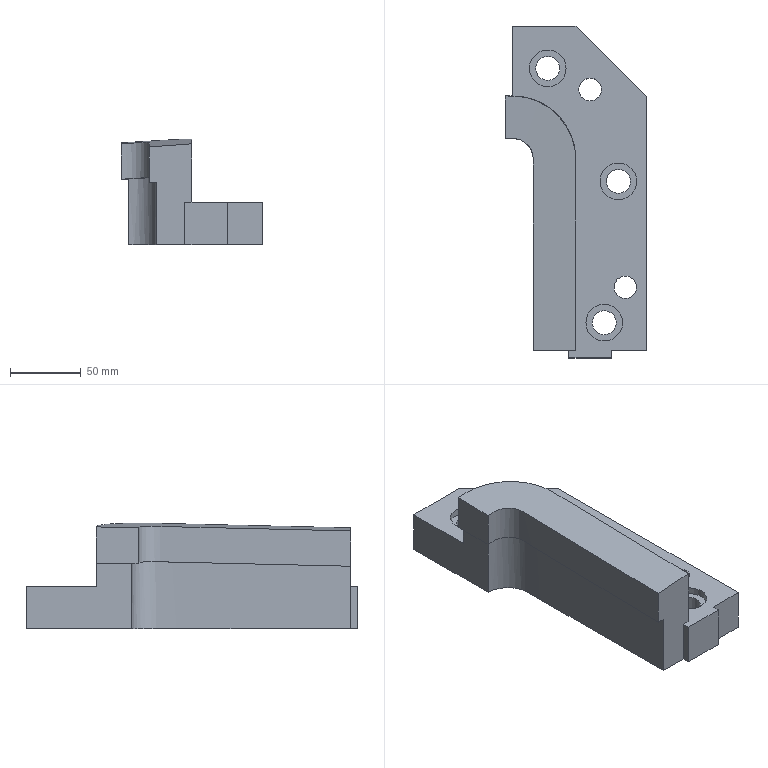Part | NX | features solid 2 | 1 solid | 30 faces | box 100.003 x 235 x 74.783 mm | volume 714230 mm3 | plane 17 | cylinder 8 | spline 5 | commonest cylinder face diameters 17 x3 26 x3 16 x2
STEP:
#1=CARTESIAN_POINT('',(660.,40.,-10.));
#2=VERTEX_POINT('',#1);
#3=CARTESIAN_POINT('',(635.,40.,-10.));
#4=VERTEX_POINT('',#3);
#5=CARTESIAN_POINT('',(660.,40.,-10.));
#6=DIRECTION('',(-1.,0.,0.));
#7=VECTOR('',#6,1000.);
#8=LINE('',#5,#7);
#9=EDGE_CURVE('',#2,#4,#8,.T.);
#10=ORIENTED_EDGE('',*,*,#9,.T.);
#11=CARTESIAN_POINT('',(635.,40.,-40.));
#12=VERTEX_POINT('',#11);
#13=CARTESIAN_POINT('',(635.,40.,-40.));
#14=DIRECTION('',(0.,0.,-1.));
#15=VECTOR('',#14,1000.);
#16=LINE('',#13,#15);
#17=EDGE_CURVE('',#12,#4,#16,.F.);
#18=ORIENTED_EDGE('',*,*,#17,.F.);
#19=CARTESIAN_POINT('',(660.,40.,-40.));
#20=VERTEX_POINT('',#19);
#21=CARTESIAN_POINT('',(609.794,40.,-40.));
#22=DIRECTION('',(-1.,0.,0.));
#23=VECTOR('',#22,1000.);
#24=LINE('',#21,#23);
#25=EDGE_CURVE('',#20,#12,#24,.T.);
#26=ORIENTED_EDGE('',*,*,#25,.F.);
#27=CARTESIAN_POINT('',(660.,40.,-300.));
#28=DIRECTION('',(0.,0.,-1.));
#29=VECTOR('',#28,1000.);
#30=LINE('',#27,#29);
#31=EDGE_CURVE('',#2,#20,#30,.T.);
#32=ORIENTED_EDGE('',*,*,#31,.F.);
#33=EDGE_LOOP('',(#10,#18,#26,#32));
#34=FACE_BOUND('',#33,.T.);
#35=CARTESIAN_POINT('',(609.803,40.,-300.));
#36=DIRECTION('',(0.,-1.,0.));
#37=DIRECTION('',(0.,0.,-1.));
#38=AXIS2_PLACEMENT_3D('',#35,#36,#37);
#39=PLANE('',#38);
#40=ADVANCED_FACE('',(#34),#39,.T.);
#41=CARTESIAN_POINT('',(605.,40.,-40.));
#42=VERTEX_POINT('',#41);
#43=CARTESIAN_POINT('',(584.803,40.,-40.));
#44=VERTEX_POINT('',#43);
#45=CARTESIAN_POINT('',(609.794,40.,-40.));
#46=DIRECTION('',(-1.,0.,0.));
#47=VECTOR('',#46,1000.);
#48=LINE('',#45,#47);
#49=EDGE_CURVE('',#42,#44,#48,.T.);
#50=ORIENTED_EDGE('',*,*,#49,.F.);
#51=CARTESIAN_POINT('',(605.,40.,-10.));
#52=VERTEX_POINT('',#51);
#53=CARTESIAN_POINT('',(605.,40.,-40.));
#54=DIRECTION('',(0.,0.,1.));
#55=VECTOR('',#54,1000.);
#56=LINE('',#53,#55);
#57=EDGE_CURVE('',#42,#52,#56,.T.);
#58=ORIENTED_EDGE('',*,*,#57,.T.);
#59=CARTESIAN_POINT('',(609.803,40.,-10.));
#60=VERTEX_POINT('',#59);
#61=CARTESIAN_POINT('',(609.803,40.,-10.));
#62=DIRECTION('',(-1.,0.,0.));
#63=VECTOR('',#62,1000.);
#64=LINE('',#61,#63);
#65=EDGE_CURVE('',#52,#60,#64,.F.);
#66=ORIENTED_EDGE('',*,*,#65,.T.);
#67=CARTESIAN_POINT('',(609.803,40.,31.479));
#68=VERTEX_POINT('',#67);
#69=CARTESIAN_POINT('',(609.803,40.,-300.));
#70=DIRECTION('',(0.,0.,1.));
#71=VECTOR('',#70,1000.);
#72=LINE('',#69,#71);
#73=EDGE_CURVE('',#60,#68,#72,.T.);
#74=ORIENTED_EDGE('',*,*,#73,.T.);
#75=CARTESIAN_POINT('',(579.803,40.,29.317));
#76=VERTEX_POINT('',#75);
#77=CARTESIAN_POINT('',(609.803,40.,31.479));
#78=CARTESIAN_POINT('',(599.805,40.,30.733));
#79=CARTESIAN_POINT('',(589.805,40.,30.013));
#80=CARTESIAN_POINT('',(579.803,40.,29.317));
#81=B_SPLINE_CURVE_WITH_KNOTS('',3,(#77,#78,#79,#80),.UNSPECIFIED.,.F.,.F.,(4,4),(0.,0.03008),.UNSPECIFIED.);
#82=EDGE_CURVE('',#68,#76,#81,.T.);
#83=ORIENTED_EDGE('',*,*,#82,.T.);
#84=CARTESIAN_POINT('',(579.803,40.,4.317));
#85=VERTEX_POINT('',#84);
#86=CARTESIAN_POINT('',(579.803,40.,-300.));
#87=DIRECTION('',(0.,0.,1.));
#88=VECTOR('',#87,1000.);
#89=LINE('',#86,#88);
#90=EDGE_CURVE('',#85,#76,#89,.T.);
#91=ORIENTED_EDGE('',*,*,#90,.F.);
#92=CARTESIAN_POINT('',(584.803,40.,4.317));
#93=VERTEX_POINT('',#92);
#94=CARTESIAN_POINT('',(584.803,40.,4.317));
#95=CARTESIAN_POINT('',(583.136,40.,4.317));
#96=CARTESIAN_POINT('',(581.47,40.,4.317));
#97=CARTESIAN_POINT('',(579.803,40.,4.317));
#98=B_SPLINE_CURVE_WITH_KNOTS('',3,(#94,#95,#96,#97),.UNSPECIFIED.,.F.,.F.,(4,4),(0.,0.005),.UNSPECIFIED.);
#99=EDGE_CURVE('',#93,#85,#98,.T.);
#100=ORIENTED_EDGE('',*,*,#99,.F.);
#101=CARTESIAN_POINT('',(584.803,40.,-145.683));
#102=DIRECTION('',(0.,0.,-1.));
#103=VECTOR('',#102,1000.);
#104=LINE('',#101,#103);
#105=EDGE_CURVE('',#44,#93,#104,.F.);
#106=ORIENTED_EDGE('',*,*,#105,.F.);
#107=EDGE_LOOP('',(#50,#58,#66,#74,#83,#91,#100,#106));
#108=FACE_BOUND('',#107,.T.);
#109=CARTESIAN_POINT('',(609.803,40.,-300.));
#110=DIRECTION('',(0.,-1.,0.));
#111=DIRECTION('',(0.,0.,-1.));
#112=AXIS2_PLACEMENT_3D('',#109,#110,#111);
#113=PLANE('',#112);
#114=ADVANCED_FACE('',(#108),#113,.T.);
#115=CARTESIAN_POINT('',(598.5,240.,-40.));
#116=VERTEX_POINT('',#115);
#117=CARTESIAN_POINT('',(590.,240.,-40.));
#118=DIRECTION('',(0.,0.,1.));
#119=DIRECTION('',(1.,0.,0.));
#120=AXIS2_PLACEMENT_3D('',#117,#118,#119);
#121=CIRCLE('',#120,8.5);
#122=EDGE_CURVE('',#116,#116,#121,.T.);
#123=ORIENTED_EDGE('',*,*,#122,.T.);
#124=EDGE_LOOP('',(#123));
#125=FACE_BOUND('',#124,.T.);
#126=CARTESIAN_POINT('',(648.5,160.,-40.));
#127=VERTEX_POINT('',#126);
#128=CARTESIAN_POINT('',(640.,160.,-40.));
#129=DIRECTION('',(0.,0.,1.));
#130=DIRECTION('',(1.,0.,0.));
#131=AXIS2_PLACEMENT_3D('',#128,#129,#130);
#132=CIRCLE('',#131,8.5);
#133=EDGE_CURVE('',#127,#127,#132,.T.);
#134=ORIENTED_EDGE('',*,*,#133,.T.);
#135=EDGE_LOOP('',(#134));
#136=FACE_BOUND('',#135,.T.);
#137=CARTESIAN_POINT('',(638.5,60.,-40.));
#138=VERTEX_POINT('',#137);
#139=CARTESIAN_POINT('',(630.,60.,-40.));
#140=DIRECTION('',(0.,0.,1.));
#141=DIRECTION('',(1.,0.,0.));
#142=AXIS2_PLACEMENT_3D('',#139,#140,#141);
#143=CIRCLE('',#142,8.5);
#144=EDGE_CURVE('',#138,#138,#143,.T.);
#145=ORIENTED_EDGE('',*,*,#144,.T.);
#146=EDGE_LOOP('',(#145));
#147=FACE_BOUND('',#146,.T.);
#148=CARTESIAN_POINT('',(628.,225.,-40.));
#149=VERTEX_POINT('',#148);
#150=CARTESIAN_POINT('',(620.,225.,-40.));
#151=DIRECTION('',(0.,0.,1.));
#152=DIRECTION('',(1.,0.,0.));
#153=AXIS2_PLACEMENT_3D('',#150,#151,#152);
#154=CIRCLE('',#153,8.);
#155=EDGE_CURVE('',#149,#149,#154,.T.);
#156=ORIENTED_EDGE('',*,*,#155,.T.);
#157=EDGE_LOOP('',(#156));
#158=FACE_BOUND('',#157,.T.);
#159=CARTESIAN_POINT('',(653.,85.,-40.));
#160=VERTEX_POINT('',#159);
#161=CARTESIAN_POINT('',(645.,85.,-40.));
#162=DIRECTION('',(0.,0.,1.));
#163=DIRECTION('',(1.,0.,0.));
#164=AXIS2_PLACEMENT_3D('',#161,#162,#163);
#165=CIRCLE('',#164,8.);
#166=EDGE_CURVE('',#160,#160,#165,.T.);
#167=ORIENTED_EDGE('',*,*,#166,.T.);
#168=EDGE_LOOP('',(#167));
#169=FACE_BOUND('',#168,.T.);
#170=CARTESIAN_POINT('',(605.,35.,-40.));
#171=VERTEX_POINT('',#170);
#172=CARTESIAN_POINT('',(605.,40.,-40.));
#173=DIRECTION('',(0.,-1.,0.));
#174=VECTOR('',#173,1000.);
#175=LINE('',#172,#174);
#176=EDGE_CURVE('',#42,#171,#175,.T.);
#177=ORIENTED_EDGE('',*,*,#176,.F.);
#178=ORIENTED_EDGE('',*,*,#49,.T.);
#179=CARTESIAN_POINT('',(565.,195.391,-40.));
#180=VERTEX_POINT('',#179);
#181=CARTESIAN_POINT('',(584.803,40.,-40.));
#182=CARTESIAN_POINT('',(584.801,46.951,-40.));
#183=CARTESIAN_POINT('',(584.798,60.853,-40.));
#184=CARTESIAN_POINT('',(584.793,81.705,-40.));
#185=CARTESIAN_POINT('',(584.79,102.558,-40.));
#186=CARTESIAN_POINT('',(584.792,119.935,-40.));
#187=CARTESIAN_POINT('',(584.798,133.836,-40.));
#188=CARTESIAN_POINT('',(584.805,144.263,-40.));
#189=CARTESIAN_POINT('',(584.816,152.951,-40.));
#190=CARTESIAN_POINT('',(584.821,159.902,-40.));
#191=CARTESIAN_POINT('',(584.836,165.116,-40.));
#192=CARTESIAN_POINT('',(584.814,170.326,-40.));
#193=CARTESIAN_POINT('',(584.936,175.551,-40.));
#194=CARTESIAN_POINT('',(584.369,180.719,-40.));
#195=CARTESIAN_POINT('',(582.328,185.559,-40.));
#196=CARTESIAN_POINT('',(579.143,189.697,-40.));
#197=CARTESIAN_POINT('',(575.018,192.889,-40.));
#198=CARTESIAN_POINT('',(570.21,194.925,-40.));
#199=CARTESIAN_POINT('',(566.731,195.341,-40.));
#200=CARTESIAN_POINT('',(565.,195.391,-40.));
#201=B_SPLINE_CURVE_WITH_KNOTS('',3,(#181,#182,#183,#184,#185,#186,#187,#188,#189,#190,#191,#192,#193,#194,#195,#196,#197,#198,#199,#200),.UNSPECIFIED.,.F.,.F.,(4,1,1,1,1,1,1,1,1,1,1,1,1,1,1,1,1,4),(0.,0.02085,0.04171,0.06256,0.08341,0.09384,0.1043,0.1147,0.1199,0.1251,0.1303,0.1355,0.1408,0.146,0.1512,0.1564,0.1616,0.1668),.UNSPECIFIED.);
#202=EDGE_CURVE('',#44,#180,#201,.T.);
#203=ORIENTED_EDGE('',*,*,#202,.T.);
#204=CARTESIAN_POINT('',(565.,270.,-40.));
#205=VERTEX_POINT('',#204);
#206=CARTESIAN_POINT('',(565.,121.934,-40.));
#207=DIRECTION('',(0.,-1.,0.));
#208=VECTOR('',#207,1000.);
#209=LINE('',#206,#208);
#210=EDGE_CURVE('',#205,#180,#209,.T.);
#211=ORIENTED_EDGE('',*,*,#210,.F.);
#212=CARTESIAN_POINT('',(610.,270.,-40.));
#213=VERTEX_POINT('',#212);
#214=CARTESIAN_POINT('',(660.,270.,-40.));
#215=DIRECTION('',(-1.,0.,0.));
#216=VECTOR('',#215,1000.);
#217=LINE('',#214,#216);
#218=EDGE_CURVE('',#213,#205,#217,.T.);
#219=ORIENTED_EDGE('',*,*,#218,.F.);
#220=CARTESIAN_POINT('',(660.,220.,-40.));
#221=VERTEX_POINT('',#220);
#222=CARTESIAN_POINT('',(660.,220.,-40.));
#223=DIRECTION('',(0.7071,-0.7071,0.));
#224=VECTOR('',#223,1000.);
#225=LINE('',#222,#224);
#226=EDGE_CURVE('',#221,#213,#225,.F.);
#227=ORIENTED_EDGE('',*,*,#226,.F.);
#228=CARTESIAN_POINT('',(660.,-215.,-40.));
#229=DIRECTION('',(0.,1.,0.));
#230=VECTOR('',#229,1000.);
#231=LINE('',#228,#230);
#232=EDGE_CURVE('',#20,#221,#231,.T.);
#233=ORIENTED_EDGE('',*,*,#232,.F.);
#234=ORIENTED_EDGE('',*,*,#25,.T.);
#235=CARTESIAN_POINT('',(635.,35.,-40.));
#236=VERTEX_POINT('',#235);
#237=CARTESIAN_POINT('',(635.,40.,-40.));
#238=DIRECTION('',(0.,1.,0.));
#239=VECTOR('',#238,1000.);
#240=LINE('',#237,#239);
#241=EDGE_CURVE('',#12,#236,#240,.F.);
#242=ORIENTED_EDGE('',*,*,#241,.T.);
#243=CARTESIAN_POINT('',(645.,35.,-40.));
#244=DIRECTION('',(1.,0.,0.));
#245=VECTOR('',#244,1000.);
#246=LINE('',#243,#245);
#247=EDGE_CURVE('',#236,#171,#246,.F.);
#248=ORIENTED_EDGE('',*,*,#247,.T.);
#249=EDGE_LOOP('',(#177,#178,#203,#211,#219,#227,#233,#234,#242,#248));
#250=FACE_BOUND('',#249,.T.);
#251=CARTESIAN_POINT('',(609.794,121.934,-40.));
#252=DIRECTION('',(0.,0.,1.));
#253=DIRECTION('',(-1.,0.,0.));
#254=AXIS2_PLACEMENT_3D('',#251,#252,#253);
#255=PLANE('',#254);
#256=ADVANCED_FACE('',(#125,#136,#147,#158,#169,#250),#255,.F.);
#257=CARTESIAN_POINT('',(603.,240.,-10.));
#258=VERTEX_POINT('',#257);
#259=CARTESIAN_POINT('',(590.,240.,-10.));
#260=DIRECTION('',(0.,0.,1.));
#261=DIRECTION('',(1.,0.,0.));
#262=AXIS2_PLACEMENT_3D('',#259,#260,#261);
#263=CIRCLE('',#262,13.);
#264=EDGE_CURVE('',#258,#258,#263,.T.);
#265=ORIENTED_EDGE('',*,*,#264,.F.);
#266=EDGE_LOOP('',(#265));
#267=FACE_BOUND('',#266,.T.);
#268=CARTESIAN_POINT('',(653.,160.,-10.));
#269=VERTEX_POINT('',#268);
#270=CARTESIAN_POINT('',(640.,160.,-10.));
#271=DIRECTION('',(0.,0.,1.));
#272=DIRECTION('',(1.,0.,0.));
#273=AXIS2_PLACEMENT_3D('',#270,#271,#272);
#274=CIRCLE('',#273,13.);
#275=EDGE_CURVE('',#269,#269,#274,.T.);
#276=ORIENTED_EDGE('',*,*,#275,.F.);
#277=EDGE_LOOP('',(#276));
#278=FACE_BOUND('',#277,.T.);
#279=CARTESIAN_POINT('',(643.,60.,-10.));
#280=VERTEX_POINT('',#279);
#281=CARTESIAN_POINT('',(630.,60.,-10.));
#282=DIRECTION('',(0.,0.,1.));
#283=DIRECTION('',(1.,0.,0.));
#284=AXIS2_PLACEMENT_3D('',#281,#282,#283);
#285=CIRCLE('',#284,13.);
#286=EDGE_CURVE('',#280,#280,#285,.T.);
#287=ORIENTED_EDGE('',*,*,#286,.F.);
#288=EDGE_LOOP('',(#287));
#289=FACE_BOUND('',#288,.T.);
#290=CARTESIAN_POINT('',(628.,225.,-10.));
#291=VERTEX_POINT('',#290);
#292=CARTESIAN_POINT('',(620.,225.,-10.));
#293=DIRECTION('',(0.,0.,1.));
#294=DIRECTION('',(1.,0.,0.));
#295=AXIS2_PLACEMENT_3D('',#292,#293,#294);
#296=CIRCLE('',#295,8.);
#297=EDGE_CURVE('',#291,#291,#296,.T.);
#298=ORIENTED_EDGE('',*,*,#297,.F.);
#299=EDGE_LOOP('',(#298));
#300=FACE_BOUND('',#299,.T.);
#301=CARTESIAN_POINT('',(653.,85.,-10.));
#302=VERTEX_POINT('',#301);
#303=CARTESIAN_POINT('',(645.,85.,-10.));
#304=DIRECTION('',(0.,0.,1.));
#305=DIRECTION('',(1.,0.,0.));
#306=AXIS2_PLACEMENT_3D('',#303,#304,#305);
#307=CIRCLE('',#306,8.);
#308=EDGE_CURVE('',#302,#302,#307,.T.);
#309=ORIENTED_EDGE('',*,*,#308,.F.);
#310=EDGE_LOOP('',(#309));
#311=FACE_BOUND('',#310,.T.);
#312=CARTESIAN_POINT('',(635.,35.,-10.));
#313=VERTEX_POINT('',#312);
#314=CARTESIAN_POINT('',(635.,40.,-10.));
#315=DIRECTION('',(0.,-1.,0.));
#316=VECTOR('',#315,1000.);
#317=LINE('',#314,#316);
#318=EDGE_CURVE('',#4,#313,#317,.T.);
#319=ORIENTED_EDGE('',*,*,#318,.F.);
#320=ORIENTED_EDGE('',*,*,#9,.F.);
#321=CARTESIAN_POINT('',(660.,220.,-10.));
#322=VERTEX_POINT('',#321);
#323=CARTESIAN_POINT('',(660.,-215.,-10.));
#324=DIRECTION('',(0.,1.,0.));
#325=VECTOR('',#324,1000.);
#326=LINE('',#323,#325);
#327=EDGE_CURVE('',#2,#322,#326,.T.);
#328=ORIENTED_EDGE('',*,*,#327,.T.);
#329=CARTESIAN_POINT('',(610.,270.,-10.));
#330=VERTEX_POINT('',#329);
#331=CARTESIAN_POINT('',(877.5,2.5,-10.));
#332=DIRECTION('',(-0.7071,0.7071,0.));
#333=VECTOR('',#332,1000.);
#334=LINE('',#331,#333);
#335=EDGE_CURVE('',#330,#322,#334,.F.);
#336=ORIENTED_EDGE('',*,*,#335,.F.);
#337=CARTESIAN_POINT('',(565.,270.,-10.));
#338=VERTEX_POINT('',#337);
#339=CARTESIAN_POINT('',(660.,270.,-10.));
#340=DIRECTION('',(-1.,0.,0.));
#341=VECTOR('',#340,1000.);
#342=LINE('',#339,#341);
#343=EDGE_CURVE('',#330,#338,#342,.T.);
#344=ORIENTED_EDGE('',*,*,#343,.T.);
#345=CARTESIAN_POINT('',(565.,220.388,-10.));
#346=VERTEX_POINT('',#345);
#347=CARTESIAN_POINT('',(565.,-215.,-10.));
#348=DIRECTION('',(0.,-1.,0.));
#349=VECTOR('',#348,1000.);
#350=LINE('',#347,#349);
#351=EDGE_CURVE('',#338,#346,#350,.T.);
#352=ORIENTED_EDGE('',*,*,#351,.T.);
#353=CARTESIAN_POINT('',(609.803,40.,-10.));
#354=CARTESIAN_POINT('',(609.797,67.324,-10.));
#355=CARTESIAN_POINT('',(609.766,108.793,-10.));
#356=CARTESIAN_POINT('',(609.827,152.054,-10.));
#357=CARTESIAN_POINT('',(609.828,170.484,-10.));
#358=CARTESIAN_POINT('',(609.852,174.233,-10.));
#359=CARTESIAN_POINT('',(609.824,176.995,-10.));
#360=CARTESIAN_POINT('',(609.6,180.207,-10.));
#361=CARTESIAN_POINT('',(608.89,185.117,-10.));
#362=CARTESIAN_POINT('',(607.115,191.421,-10.));
#363=CARTESIAN_POINT('',(603.789,198.368,-10.));
#364=CARTESIAN_POINT('',(599.387,204.588,-10.));
#365=CARTESIAN_POINT('',(593.924,210.044,-10.));
#366=CARTESIAN_POINT('',(587.673,214.455,-10.));
#367=CARTESIAN_POINT('',(580.59,217.807,-10.));
#368=CARTESIAN_POINT('',(573.327,219.802,-10.));
#369=CARTESIAN_POINT('',(568.272,220.327,-10.));
#370=CARTESIAN_POINT('',(565.167,220.389,-10.));
#371=CARTESIAN_POINT('',(564.525,220.39,-10.));
#372=CARTESIAN_POINT('',(563.605,220.383,-10.));
#373=CARTESIAN_POINT('',(562.153,220.388,-10.));
#374=CARTESIAN_POINT('',(560.855,220.386,-10.));
#375=CARTESIAN_POINT('',(560.,220.386,-10.));
#376=B_SPLINE_CURVE_WITH_KNOTS('',3,(#353,#354,#355,#356,#357,#358,#359,#360,#361,#362,#363,#364,#365,#366,#367,#368,#369,#370,#371,#372,#373,#374,#375),.UNSPECIFIED.,.F.,.F.,(4,1,1,1,1,1,1,1,1,1,1,1,1,1,1,1,1,1,1,1,4),(0.,0.5,0.75,0.8125,0.8203,0.8281,0.8359,0.8437,0.8594,0.875,0.8906,0.9062,0.9218,0.9375,0.9531,0.9677,0.9687,0.9726,0.9765,0.9843,1.),.UNSPECIFIED.);
#377=EDGE_CURVE('',#346,#60,#376,.F.);
#378=ORIENTED_EDGE('',*,*,#377,.T.);
#379=ORIENTED_EDGE('',*,*,#65,.F.);
#380=CARTESIAN_POINT('',(605.,35.,-10.));
#381=VERTEX_POINT('',#380);
#382=CARTESIAN_POINT('',(605.,40.,-10.));
#383=DIRECTION('',(0.,1.,0.));
#384=VECTOR('',#383,1000.);
#385=LINE('',#382,#384);
#386=EDGE_CURVE('',#52,#381,#385,.F.);
#387=ORIENTED_EDGE('',*,*,#386,.T.);
#388=CARTESIAN_POINT('',(645.,35.,-10.));
#389=DIRECTION('',(1.,0.,0.));
#390=VECTOR('',#389,1000.);
#391=LINE('',#388,#390);
#392=EDGE_CURVE('',#313,#381,#391,.F.);
#393=ORIENTED_EDGE('',*,*,#392,.F.);
#394=EDGE_LOOP('',(#319,#320,#328,#336,#344,#352,#378,#379,#387,#393));
#395=FACE_BOUND('',#394,.T.);
#396=CARTESIAN_POINT('',(660.,-215.,-10.));
#397=DIRECTION('',(0.,0.,1.));
#398=DIRECTION('',(0.,1.,0.));
#399=AXIS2_PLACEMENT_3D('',#396,#397,#398);
#400=PLANE('',#399);
#401=ADVANCED_FACE('',(#267,#278,#289,#300,#311,#395),#400,.T.);
#402=CARTESIAN_POINT('',(560.,220.386,6.411));
#403=VERTEX_POINT('',#402);
#404=CARTESIAN_POINT('',(565.,220.388,6.411));
#405=VERTEX_POINT('',#404);
#406=CARTESIAN_POINT('',(609.803,40.,6.411));
#407=CARTESIAN_POINT('',(609.797,67.324,6.411));
#408=CARTESIAN_POINT('',(609.766,108.793,6.411));
#409=CARTESIAN_POINT('',(609.827,152.054,6.411));
#410=CARTESIAN_POINT('',(609.828,170.484,6.411));
#411=CARTESIAN_POINT('',(609.852,174.233,6.411));
#412=CARTESIAN_POINT('',(609.824,176.995,6.411));
#413=CARTESIAN_POINT('',(609.6,180.207,6.411));
#414=CARTESIAN_POINT('',(608.89,185.117,6.411));
#415=CARTESIAN_POINT('',(607.115,191.421,6.411));
#416=CARTESIAN_POINT('',(603.789,198.368,6.411));
#417=CARTESIAN_POINT('',(599.387,204.588,6.411));
#418=CARTESIAN_POINT('',(593.924,210.044,6.411));
#419=CARTESIAN_POINT('',(587.673,214.455,6.411));
#420=CARTESIAN_POINT('',(580.59,217.807,6.411));
#421=CARTESIAN_POINT('',(573.327,219.802,6.411));
#422=CARTESIAN_POINT('',(568.272,220.327,6.411));
#423=CARTESIAN_POINT('',(565.167,220.389,6.411));
#424=CARTESIAN_POINT('',(564.525,220.39,6.411));
#425=CARTESIAN_POINT('',(563.605,220.383,6.411));
#426=CARTESIAN_POINT('',(562.153,220.388,6.411));
#427=CARTESIAN_POINT('',(560.855,220.386,6.411));
#428=CARTESIAN_POINT('',(560.,220.386,6.411));
#429=B_SPLINE_CURVE_WITH_KNOTS('',3,(#406,#407,#408,#409,#410,#411,#412,#413,#414,#415,#416,#417,#418,#419,#420,#421,#422,#423,#424,#425,#426,#427,#428),.UNSPECIFIED.,.F.,.F.,(4,1,1,1,1,1,1,1,1,1,1,1,1,1,1,1,1,1,1,1,4),(0.,0.5,0.75,0.8125,0.8203,0.8281,0.8359,0.8437,0.8594,0.875,0.8906,0.9062,0.9218,0.9375,0.9531,0.9677,0.9687,0.9726,0.9765,0.9843,1.),.UNSPECIFIED.);
#430=EDGE_CURVE('',#403,#405,#429,.F.);
#431=ORIENTED_EDGE('',*,*,#430,.F.);
#432=CARTESIAN_POINT('',(560.,220.386,32.162));
#433=VERTEX_POINT('',#432);
#434=CARTESIAN_POINT('',(560.,220.386,-300.));
#435=DIRECTION('',(0.,0.,1.));
#436=VECTOR('',#435,1000.);
#437=LINE('',#434,#436);
#438=EDGE_CURVE('',#403,#433,#437,.T.);
#439=ORIENTED_EDGE('',*,*,#438,.T.);
#440=CARTESIAN_POINT('',(609.803,40.,31.479));
#441=CARTESIAN_POINT('',(609.801,48.812,31.683));
#442=CARTESIAN_POINT('',(609.794,66.437,32.092));
#443=CARTESIAN_POINT('',(609.785,92.875,32.705));
#444=CARTESIAN_POINT('',(609.788,114.906,33.217));
#445=CARTESIAN_POINT('',(609.803,132.531,33.627));
#446=CARTESIAN_POINT('',(609.815,145.75,33.935));
#447=CARTESIAN_POINT('',(609.826,156.765,34.191));
#448=CARTESIAN_POINT('',(609.825,165.579,34.396));
#449=CARTESIAN_POINT('',(609.842,172.184,34.551));
#450=CARTESIAN_POINT('',(609.852,178.808,34.705));
#451=CARTESIAN_POINT('',(608.888,185.257,34.783));
#452=CARTESIAN_POINT('',(606.977,191.607,34.788));
#453=CARTESIAN_POINT('',(604.197,197.54,34.721));
#454=CARTESIAN_POINT('',(600.586,203.017,34.583));
#455=CARTESIAN_POINT('',(596.16,207.944,34.376));
#456=CARTESIAN_POINT('',(591.163,212.123,34.113));
#457=CARTESIAN_POINT('',(585.484,215.58,33.791));
#458=CARTESIAN_POINT('',(579.498,218.127,33.431));
#459=CARTESIAN_POINT('',(573.089,219.808,33.028));
#460=CARTESIAN_POINT('',(566.568,220.498,32.602));
#461=CARTESIAN_POINT('',(562.187,220.386,32.307));
#462=CARTESIAN_POINT('',(560.,220.386,32.162));
#463=B_SPLINE_CURVE_WITH_KNOTS('',3,(#440,#441,#442,#443,#444,#445,#446,#447,#448,#449,#450,#451,#452,#453,#454,#455,#456,#457,#458,#459,#460,#461,#462),.UNSPECIFIED.,.F.,.F.,(4,1,1,1,1,1,1,1,1,1,1,1,1,1,1,1,1,1,1,1,4),(0.,0.02644,0.05289,0.07933,0.09256,0.1058,0.119,0.1256,0.1322,0.1388,0.1454,0.1521,0.1587,0.1653,0.1719,0.1785,0.1851,0.1917,0.1983,0.2049,0.2116),.UNSPECIFIED.);
#464=EDGE_CURVE('',#68,#433,#463,.T.);
#465=ORIENTED_EDGE('',*,*,#464,.F.);
#466=ORIENTED_EDGE('',*,*,#73,.F.);
#467=ORIENTED_EDGE('',*,*,#377,.F.);
#468=CARTESIAN_POINT('',(565.,220.388,12.531));
#469=DIRECTION('',(0.,0.,1.));
#470=VECTOR('',#469,1000.);
#471=LINE('',#468,#470);
#472=EDGE_CURVE('',#405,#346,#471,.F.);
#473=ORIENTED_EDGE('',*,*,#472,.F.);
#474=EDGE_LOOP('',(#431,#439,#465,#466,#467,#473));
#475=FACE_BOUND('',#474,.T.);
#476=CARTESIAN_POINT('',(609.803,40.,-10.));
#477=CARTESIAN_POINT('',(609.803,40.,35.062));
#478=CARTESIAN_POINT('',(609.798,63.909,-10.));
#479=CARTESIAN_POINT('',(609.798,63.909,35.062));
#480=CARTESIAN_POINT('',(609.779,91.515,-10.));
#481=CARTESIAN_POINT('',(609.779,91.515,35.062));
#482=CARTESIAN_POINT('',(609.796,127.017,-10.));
#483=CARTESIAN_POINT('',(609.796,127.017,35.062));
#484=CARTESIAN_POINT('',(609.811,140.392,-10.));
#485=CARTESIAN_POINT('',(609.811,140.392,35.062));
#486=CARTESIAN_POINT('',(609.821,152.406,-10.));
#487=CARTESIAN_POINT('',(609.821,152.406,35.062));
#488=CARTESIAN_POINT('',(609.824,156.744,-10.));
#489=CARTESIAN_POINT('',(609.824,156.744,35.062));
#490=CARTESIAN_POINT('',(609.826,160.248,-10.));
#491=CARTESIAN_POINT('',(609.826,160.248,35.062));
#492=CARTESIAN_POINT('',(609.827,162.895,-10.));
#493=CARTESIAN_POINT('',(609.827,162.895,35.062));
#494=CARTESIAN_POINT('',(609.828,165.562,-10.));
#495=CARTESIAN_POINT('',(609.828,165.562,35.062));
#496=CARTESIAN_POINT('',(609.83,168.194,-10.));
#497=CARTESIAN_POINT('',(609.83,168.194,35.062));
#498=CARTESIAN_POINT('',(609.834,170.313,-10.));
#499=CARTESIAN_POINT('',(609.834,170.313,35.062));
#500=CARTESIAN_POINT('',(609.84,171.936,-10.));
#501=CARTESIAN_POINT('',(609.84,171.936,35.062));
#502=CARTESIAN_POINT('',(609.845,173.11,-10.));
#503=CARTESIAN_POINT('',(609.845,173.11,35.062));
#504=CARTESIAN_POINT('',(609.852,174.237,-10.));
#505=CARTESIAN_POINT('',(609.852,174.237,35.062));
#506=CARTESIAN_POINT('',(609.824,177.003,-10.));
#507=CARTESIAN_POINT('',(609.824,177.003,35.062));
#508=CARTESIAN_POINT('',(609.599,180.216,-10.));
#509=CARTESIAN_POINT('',(609.599,180.216,35.062));
#510=CARTESIAN_POINT('',(608.888,185.127,-10.));
#511=CARTESIAN_POINT('',(608.888,185.127,35.062));
#512=CARTESIAN_POINT('',(607.111,191.431,-10.));
#513=CARTESIAN_POINT('',(607.111,191.431,35.062));
#514=CARTESIAN_POINT('',(603.783,198.377,-10.));
#515=CARTESIAN_POINT('',(603.783,198.377,35.062));
#516=CARTESIAN_POINT('',(599.379,204.596,-10.));
#517=CARTESIAN_POINT('',(599.379,204.596,35.062));
#518=CARTESIAN_POINT('',(593.914,210.052,-10.));
#519=CARTESIAN_POINT('',(593.914,210.052,35.062));
#520=CARTESIAN_POINT('',(587.662,214.461,-10.));
#521=CARTESIAN_POINT('',(587.662,214.461,35.062));
#522=CARTESIAN_POINT('',(581.758,217.253,-10.));
#523=CARTESIAN_POINT('',(581.758,217.253,35.062));
#524=CARTESIAN_POINT('',(576.868,218.83,-10.));
#525=CARTESIAN_POINT('',(576.868,218.83,35.062));
#526=CARTESIAN_POINT('',(573.76,219.543,-10.));
#527=CARTESIAN_POINT('',(573.76,219.543,35.062));
#528=CARTESIAN_POINT('',(571.251,219.953,-10.));
#529=CARTESIAN_POINT('',(571.251,219.953,35.062));
#530=CARTESIAN_POINT('',(569.369,220.179,-10.));
#531=CARTESIAN_POINT('',(569.369,220.179,35.062));
#532=CARTESIAN_POINT('',(567.793,220.301,-10.));
#533=CARTESIAN_POINT('',(567.793,220.301,35.062));
#534=CARTESIAN_POINT('',(566.562,220.359,-10.));
#535=CARTESIAN_POINT('',(566.562,220.359,35.062));
#536=CARTESIAN_POINT('',(565.248,220.389,-10.));
#537=CARTESIAN_POINT('',(565.248,220.389,35.062));
#538=CARTESIAN_POINT('',(564.514,220.39,-10.));
#539=CARTESIAN_POINT('',(564.514,220.39,35.062));
#540=CARTESIAN_POINT('',(563.603,220.383,-10.));
#541=CARTESIAN_POINT('',(563.603,220.383,35.062));
#542=CARTESIAN_POINT('',(562.563,220.386,-10.));
#543=CARTESIAN_POINT('',(562.563,220.386,35.062));
#544=CARTESIAN_POINT('',(561.286,220.387,-10.));
#545=CARTESIAN_POINT('',(561.286,220.387,35.062));
#546=CARTESIAN_POINT('',(560.427,220.386,-10.));
#547=CARTESIAN_POINT('',(560.427,220.386,35.062));
#548=CARTESIAN_POINT('',(560.,220.386,-10.));
#549=CARTESIAN_POINT('',(560.,220.386,35.062));
#550=B_SPLINE_SURFACE_WITH_KNOTS('',3,1,((#476,#477),(#478,#479),(#480,#481),(#482,#483),(#484,#485),(#486,#487),(#488,#489),(#490,#491),(#492,#493),(#494,#495),(#496,#497),(#498,#499),(#500,#501),(#502,#503),(#504,#505),(#506,#507),(#508,#509),(#510,#511),(#512,#513),(#514,#515),(#516,#517),(#518,#519),(#520,#521),(#522,#523),(#524,#525),(#526,#527),(#528,#529),(#530,#531),(#532,#533),(#534,#535),(#536,#537),(#538,#539),(#540,#541),(#542,#543),(#544,#545),(#546,#547),(#548,#549)),.UNSPECIFIED.,.F.,.F.,.F.,(4,1,1,1,1,1,1,1,1,1,1,1,1,1,1,1,1,1,1,1,1,1,1,1,1,1,1,1,1,1,1,1,1,1,4),(2,2),(0.,0.4375,0.5,0.6562,0.6875,0.7188,0.7344,0.75,0.7656,0.7812,0.7969,0.8047,0.8125,0.8203,0.8281,0.8359,0.8438,0.8594,0.875,0.8906,0.9062,0.9219,0.9375,0.9453,0.9531,0.957,0.9609,0.9648,0.9668,0.9688,0.9727,0.9766,0.9844,0.9922,1.),(0.,1.),.UNSPECIFIED.);
#551=ADVANCED_FACE('',(#475),#550,.T.);
#552=ORIENTED_EDGE('',*,*,#218,.T.);
#553=CARTESIAN_POINT('',(565.,270.,6.411));
#554=DIRECTION('',(0.,0.,-1.));
#555=VECTOR('',#554,1000.);
#556=LINE('',#553,#555);
#557=EDGE_CURVE('',#338,#205,#556,.T.);
#558=ORIENTED_EDGE('',*,*,#557,.F.);
#559=ORIENTED_EDGE('',*,*,#343,.F.);
#560=CARTESIAN_POINT('',(610.,270.,-10.));
#561=DIRECTION('',(0.,0.,1.));
#562=VECTOR('',#561,1000.);
#563=LINE('',#560,#562);
#564=EDGE_CURVE('',#213,#330,#563,.T.);
#565=ORIENTED_EDGE('',*,*,#564,.F.);
#566=EDGE_LOOP('',(#552,#558,#559,#565));
#567=FACE_BOUND('',#566,.T.);
#568=CARTESIAN_POINT('',(660.,270.,-10.));
#569=DIRECTION('',(0.,1.,0.));
#570=DIRECTION('',(0.,0.,-1.));
#571=AXIS2_PLACEMENT_3D('',#568,#569,#570);
#572=PLANE('',#571);
#573=ADVANCED_FACE('',(#567),#572,.T.);
#574=CARTESIAN_POINT('',(560.,190.386,6.411));
#575=VERTEX_POINT('',#574);
#576=CARTESIAN_POINT('',(559.997,195.387,6.411));
#577=VERTEX_POINT('',#576);
#578=CARTESIAN_POINT('',(560.,190.386,6.411));
#579=DIRECTION('',(0.,1.,0.));
#580=VECTOR('',#579,1000.);
#581=LINE('',#578,#580);
#582=EDGE_CURVE('',#575,#577,#581,.T.);
#583=ORIENTED_EDGE('',*,*,#582,.F.);
#584=CARTESIAN_POINT('',(560.,190.386,31.465));
#585=VERTEX_POINT('',#584);
#586=CARTESIAN_POINT('',(560.,190.386,-300.));
#587=DIRECTION('',(0.,0.,1.));
#588=VECTOR('',#587,1000.);
#589=LINE('',#586,#588);
#590=EDGE_CURVE('',#575,#585,#589,.T.);
#591=ORIENTED_EDGE('',*,*,#590,.T.);
#592=CARTESIAN_POINT('',(560.,190.386,31.465));
#593=CARTESIAN_POINT('',(560.,200.386,31.698));
#594=CARTESIAN_POINT('',(560.,210.386,31.93));
#595=CARTESIAN_POINT('',(560.,220.386,32.162));
#596=B_SPLINE_CURVE_WITH_KNOTS('',3,(#592,#593,#594,#595),.UNSPECIFIED.,.F.,.F.,(4,4),(0.,0.03001),.UNSPECIFIED.);
#597=EDGE_CURVE('',#585,#433,#596,.T.);
#598=ORIENTED_EDGE('',*,*,#597,.T.);
#599=ORIENTED_EDGE('',*,*,#438,.F.);
#600=CARTESIAN_POINT('',(560.,190.386,6.411));
#601=DIRECTION('',(0.,1.,0.));
#602=VECTOR('',#601,1000.);
#603=LINE('',#600,#602);
#604=EDGE_CURVE('',#577,#403,#603,.T.);
#605=ORIENTED_EDGE('',*,*,#604,.F.);
#606=EDGE_LOOP('',(#583,#591,#598,#599,#605));
#607=FACE_BOUND('',#606,.T.);
#608=CARTESIAN_POINT('',(560.,190.386,-300.));
#609=DIRECTION('',(-1.,0.,0.));
#610=DIRECTION('',(0.,0.,-1.));
#611=AXIS2_PLACEMENT_3D('',#608,#609,#610);
#612=PLANE('',#611);
#613=ADVANCED_FACE('',(#607),#612,.T.);
#614=CARTESIAN_POINT('',(579.803,40.,4.317));
#615=CARTESIAN_POINT('',(579.801,46.829,4.421));
#616=CARTESIAN_POINT('',(579.798,60.482,4.808));
#617=CARTESIAN_POINT('',(579.794,80.964,5.255));
#618=CARTESIAN_POINT('',(579.791,101.446,5.738));
#619=CARTESIAN_POINT('',(579.792,118.515,6.133));
#620=CARTESIAN_POINT('',(579.797,132.17,6.45));
#621=CARTESIAN_POINT('',(579.803,142.41,6.688));
#622=CARTESIAN_POINT('',(579.813,152.652,6.927));
#623=CARTESIAN_POINT('',(579.824,161.184,7.125));
#624=CARTESIAN_POINT('',(579.835,168.016,7.285));
#625=CARTESIAN_POINT('',(579.845,173.122,7.402));
#626=CARTESIAN_POINT('',(579.853,178.297,7.532));
#627=CARTESIAN_POINT('',(578.02,183.147,7.517));
#628=CARTESIAN_POINT('',(574.704,187.111,7.36));
#629=CARTESIAN_POINT('',(570.97,189.292,7.138));
#630=CARTESIAN_POINT('',(567.696,190.203,6.923));
#631=CARTESIAN_POINT('',(565.139,190.431,6.752));
#632=CARTESIAN_POINT('',(562.568,190.373,6.58));
#633=CARTESIAN_POINT('',(560.856,190.386,6.467));
#634=CARTESIAN_POINT('',(560.,190.386,6.411));
#635=B_SPLINE_CURVE_WITH_KNOTS('',3,(#614,#615,#616,#617,#618,#619,#620,#621,#622,#623,#624,#625,#626,#627,#628,#629,#630,#631,#632,#633,#634),.UNSPECIFIED.,.F.,.F.,(4,1,1,1,1,1,1,1,1,1,1,1,1,1,1,1,1,1,4),(0.,0.02049,0.04098,0.06146,0.08195,0.09219,0.1024,0.1127,0.1229,0.128,0.1332,0.1383,0.1434,0.1485,0.1537,0.1562,0.1588,0.1613,0.1639),.UNSPECIFIED.);
#636=EDGE_CURVE('',#85,#575,#635,.T.);
#637=ORIENTED_EDGE('',*,*,#636,.F.);
#638=ORIENTED_EDGE('',*,*,#90,.T.);
#639=CARTESIAN_POINT('',(579.803,40.,29.317));
#640=CARTESIAN_POINT('',(579.801,46.811,29.475));
#641=CARTESIAN_POINT('',(579.798,60.433,29.792));
#642=CARTESIAN_POINT('',(579.794,80.866,30.266));
#643=CARTESIAN_POINT('',(579.791,101.3,30.74));
#644=CARTESIAN_POINT('',(579.792,118.327,31.135));
#645=CARTESIAN_POINT('',(579.797,131.949,31.452));
#646=CARTESIAN_POINT('',(579.803,142.166,31.689));
#647=CARTESIAN_POINT('',(579.813,152.382,31.927));
#648=CARTESIAN_POINT('',(579.821,160.896,32.126));
#649=CARTESIAN_POINT('',(579.838,167.707,32.285));
#650=CARTESIAN_POINT('',(579.829,172.816,32.403));
#651=CARTESIAN_POINT('',(579.909,177.922,32.527));
#652=CARTESIAN_POINT('',(578.17,182.922,32.522));
#653=CARTESIAN_POINT('',(574.838,187.005,32.387));
#654=CARTESIAN_POINT('',(571.08,189.254,32.182));
#655=CARTESIAN_POINT('',(567.719,190.202,31.977));
#656=CARTESIAN_POINT('',(565.15,190.432,31.809));
#657=CARTESIAN_POINT('',(562.574,190.373,31.636));
#658=CARTESIAN_POINT('',(560.858,190.386,31.522));
#659=CARTESIAN_POINT('',(560.,190.386,31.465));
#660=B_SPLINE_CURVE_WITH_KNOTS('',3,(#639,#640,#641,#642,#643,#644,#645,#646,#647,#648,#649,#650,#651,#652,#653,#654,#655,#656,#657,#658,#659),.UNSPECIFIED.,.F.,.F.,(4,1,1,1,1,1,1,1,1,1,1,1,1,1,1,1,1,1,4),(0.,0.02044,0.04088,0.06132,0.08175,0.09197,0.1022,0.1124,0.1226,0.1277,0.1329,0.138,0.1431,0.1482,0.1533,0.1558,0.1584,0.161,0.1635),.UNSPECIFIED.);
#661=EDGE_CURVE('',#76,#585,#660,.T.);
#662=ORIENTED_EDGE('',*,*,#661,.T.);
#663=ORIENTED_EDGE('',*,*,#590,.F.);
#664=EDGE_LOOP('',(#637,#638,#662,#663));
#665=FACE_BOUND('',#664,.T.);
#666=CARTESIAN_POINT('',(579.803,40.,4.148));
#667=CARTESIAN_POINT('',(579.803,40.,32.689));
#668=CARTESIAN_POINT('',(579.801,46.83,4.148));
#669=CARTESIAN_POINT('',(579.801,46.83,32.689));
#670=CARTESIAN_POINT('',(579.798,60.49,4.148));
#671=CARTESIAN_POINT('',(579.798,60.49,32.689));
#672=CARTESIAN_POINT('',(579.794,80.98,4.148));
#673=CARTESIAN_POINT('',(579.794,80.98,32.689));
#674=CARTESIAN_POINT('',(579.791,101.47,4.148));
#675=CARTESIAN_POINT('',(579.791,101.47,32.689));
#676=CARTESIAN_POINT('',(579.792,118.545,4.148));
#677=CARTESIAN_POINT('',(579.792,118.545,32.689));
#678=CARTESIAN_POINT('',(579.797,132.205,4.148));
#679=CARTESIAN_POINT('',(579.797,132.205,32.689));
#680=CARTESIAN_POINT('',(579.803,142.449,4.148));
#681=CARTESIAN_POINT('',(579.803,142.449,32.689));
#682=CARTESIAN_POINT('',(579.813,152.695,4.148));
#683=CARTESIAN_POINT('',(579.813,152.695,32.689));
#684=CARTESIAN_POINT('',(579.824,161.23,4.148));
#685=CARTESIAN_POINT('',(579.824,161.23,32.689));
#686=CARTESIAN_POINT('',(579.834,168.064,4.148));
#687=CARTESIAN_POINT('',(579.834,168.064,32.689));
#688=CARTESIAN_POINT('',(579.847,173.175,4.148));
#689=CARTESIAN_POINT('',(579.847,173.175,32.689));
#690=CARTESIAN_POINT('',(579.847,178.34,4.148));
#691=CARTESIAN_POINT('',(579.847,178.34,32.689));
#692=CARTESIAN_POINT('',(577.991,183.196,4.148));
#693=CARTESIAN_POINT('',(577.991,183.196,32.689));
#694=CARTESIAN_POINT('',(574.673,187.132,4.148));
#695=CARTESIAN_POINT('',(574.673,187.132,32.689));
#696=CARTESIAN_POINT('',(570.966,189.295,4.148));
#697=CARTESIAN_POINT('',(570.966,189.295,32.689));
#698=CARTESIAN_POINT('',(567.676,190.208,4.148));
#699=CARTESIAN_POINT('',(567.676,190.208,32.689));
#700=CARTESIAN_POINT('',(565.121,190.431,4.148));
#701=CARTESIAN_POINT('',(565.121,190.431,32.689));
#702=CARTESIAN_POINT('',(562.56,190.373,4.148));
#703=CARTESIAN_POINT('',(562.56,190.373,32.689));
#704=CARTESIAN_POINT('',(560.853,190.386,4.148));
#705=CARTESIAN_POINT('',(560.853,190.386,32.689));
#706=CARTESIAN_POINT('',(560.,190.386,4.148));
#707=CARTESIAN_POINT('',(560.,190.386,32.689));
#708=B_SPLINE_SURFACE_WITH_KNOTS('',3,1,((#666,#667),(#668,#669),(#670,#671),(#672,#673),(#674,#675),(#676,#677),(#678,#679),(#680,#681),(#682,#683),(#684,#685),(#686,#687),(#688,#689),(#690,#691),(#692,#693),(#694,#695),(#696,#697),(#698,#699),(#700,#701),(#702,#703),(#704,#705),(#706,#707)),.SURF_OF_LINEAR_EXTRUSION.,.F.,.F.,.F.,(4,1,1,1,1,1,1,1,1,1,1,1,1,1,1,1,1,1,4),(2,2),(0.,0.125,0.25,0.375,0.5,0.5625,0.625,0.6875,0.75,0.7812,0.8125,0.8438,0.875,0.9062,0.9375,0.9531,0.9688,0.9844,1.),(0.,1.),.UNSPECIFIED.);
#709=ADVANCED_FACE('',(#665),#708,.F.);
#710=ORIENTED_EDGE('',*,*,#82,.F.);
#711=ORIENTED_EDGE('',*,*,#464,.T.);
#712=ORIENTED_EDGE('',*,*,#597,.F.);
#713=ORIENTED_EDGE('',*,*,#661,.F.);
#714=EDGE_LOOP('',(#710,#711,#712,#713));
#715=FACE_BOUND('',#714,.T.);
#716=CARTESIAN_POINT('',(610.328,221.396,35.729));
#717=CARTESIAN_POINT('',(610.328,38.867,31.492));
#718=CARTESIAN_POINT('',(593.557,221.425,34.478));
#719=CARTESIAN_POINT('',(593.557,38.896,30.24));
#720=CARTESIAN_POINT('',(576.781,221.453,33.297));
#721=CARTESIAN_POINT('',(576.781,38.923,29.059));
#722=CARTESIAN_POINT('',(560.,221.478,32.187));
#723=CARTESIAN_POINT('',(560.,38.949,27.949));
#724=(BOUNDED_SURFACE()B_SPLINE_SURFACE(3,1,((#716,#717),(#718,#719),(#720,#721),(#722,#723)),.SURF_OF_LINEAR_EXTRUSION.,.F.,.F.,.F.)B_SPLINE_SURFACE_WITH_KNOTS((4,4),(2,2),(0.1479,0.197),(0.285,0.4672),.PIECEWISE_BEZIER_KNOTS.)GEOMETRIC_REPRESENTATION_ITEM()RATIONAL_B_SPLINE_SURFACE(((0.9998,0.9998),(0.9998,0.9998),(0.9998,0.9998),(0.9998,0.9998)))REPRESENTATION_ITEM('')SURFACE());
#725=ADVANCED_FACE('',(#715),#724,.T.);
#726=CARTESIAN_POINT('',(660.,220.,-10.));
#727=DIRECTION('',(0.,0.,-1.));
#728=VECTOR('',#727,1000.);
#729=LINE('',#726,#728);
#730=EDGE_CURVE('',#322,#221,#729,.T.);
#731=ORIENTED_EDGE('',*,*,#730,.F.);
#732=ORIENTED_EDGE('',*,*,#327,.F.);
#733=ORIENTED_EDGE('',*,*,#31,.T.);
#734=ORIENTED_EDGE('',*,*,#232,.T.);
#735=EDGE_LOOP('',(#731,#732,#733,#734));
#736=FACE_BOUND('',#735,.T.);
#737=CARTESIAN_POINT('',(660.,-215.,-10.));
#738=DIRECTION('',(1.,0.,0.));
#739=DIRECTION('',(0.,0.,1.));
#740=AXIS2_PLACEMENT_3D('',#737,#738,#739);
#741=PLANE('',#740);
#742=ADVANCED_FACE('',(#736),#741,.T.);
#743=ORIENTED_EDGE('',*,*,#335,.T.);
#744=ORIENTED_EDGE('',*,*,#730,.T.);
#745=ORIENTED_EDGE('',*,*,#226,.T.);
#746=ORIENTED_EDGE('',*,*,#564,.T.);
#747=EDGE_LOOP('',(#743,#744,#745,#746));
#748=FACE_BOUND('',#747,.T.);
#749=CARTESIAN_POINT('',(660.,220.,-10.));
#750=DIRECTION('',(-0.7071,-0.7071,0.));
#751=DIRECTION('',(-0.7071,0.7071,0.));
#752=AXIS2_PLACEMENT_3D('',#749,#750,#751);
#753=PLANE('',#752);
#754=ADVANCED_FACE('',(#748),#753,.F.);
#755=ORIENTED_EDGE('',*,*,#636,.T.);
#756=CARTESIAN_POINT('',(560.,190.386,6.411));
#757=CARTESIAN_POINT('',(560.001,192.053,6.411));
#758=CARTESIAN_POINT('',(560.002,193.72,6.411));
#759=CARTESIAN_POINT('',(560.003,195.387,6.411));
#760=B_SPLINE_CURVE_WITH_KNOTS('',3,(#756,#757,#758,#759),.UNSPECIFIED.,.F.,.F.,(4,4),(0.0001873,0.005188),.UNSPECIFIED.);
#761=EDGE_CURVE('',#575,#577,#760,.T.);
#762=ORIENTED_EDGE('',*,*,#761,.T.);
#763=CARTESIAN_POINT('',(584.803,40.,4.317));
#764=CARTESIAN_POINT('',(584.801,46.827,4.421));
#765=CARTESIAN_POINT('',(584.798,60.478,4.808));
#766=CARTESIAN_POINT('',(584.793,80.956,5.255));
#767=CARTESIAN_POINT('',(584.791,98.02,5.658));
#768=CARTESIAN_POINT('',(584.791,111.671,5.974));
#769=CARTESIAN_POINT('',(584.793,121.908,6.212));
#770=CARTESIAN_POINT('',(584.798,132.146,6.45));
#771=CARTESIAN_POINT('',(584.804,142.384,6.688));
#772=CARTESIAN_POINT('',(584.812,150.915,6.887));
#773=CARTESIAN_POINT('',(584.82,157.741,7.046));
#774=CARTESIAN_POINT('',(584.826,162.86,7.165));
#775=CARTESIAN_POINT('',(584.832,167.126,7.264));
#776=CARTESIAN_POINT('',(584.838,170.534,7.344));
#777=CARTESIAN_POINT('',(584.843,172.663,7.394));
#778=CARTESIAN_POINT('',(584.849,174.395,7.434));
#779=CARTESIAN_POINT('',(584.819,175.867,7.463));
#780=CARTESIAN_POINT('',(584.726,177.393,7.489));
#781=CARTESIAN_POINT('',(584.426,179.665,7.516));
#782=CARTESIAN_POINT('',(583.656,182.459,7.525));
#783=CARTESIAN_POINT('',(581.69,186.595,7.491));
#784=CARTESIAN_POINT('',(577.974,190.99,7.36));
#785=CARTESIAN_POINT('',(573.021,193.933,7.137));
#786=CARTESIAN_POINT('',(568.515,195.157,6.921));
#787=CARTESIAN_POINT('',(565.198,195.433,6.75));
#788=CARTESIAN_POINT('',(562.448,195.399,6.579));
#789=CARTESIAN_POINT('',(560.848,195.387,6.467));
#790=CARTESIAN_POINT('',(560.,195.387,6.411));
#791=B_SPLINE_CURVE_WITH_KNOTS('',3,(#763,#764,#765,#766,#767,#768,#769,#770,#771,#772,#773,#774,#775,#776,#777,#778,#779,#780,#781,#782,#783,#784,#785,#786,#787,#788,#789,#790),.UNSPECIFIED.,.F.,.F.,(4,1,1,1,1,1,1,1,1,1,1,1,1,1,1,1,1,1,1,1,1,1,1,1,1,4),(-0.000002383,0.04505,0.0901,0.1351,0.1577,0.1802,0.2027,0.2253,0.2478,0.259,0.2703,0.2816,0.2872,0.2928,0.2956,0.2985,0.3013,0.3041,0.3097,0.3154,0.3266,0.3379,0.3435,0.3491,0.3548,0.3604),.UNSPECIFIED.);
#792=EDGE_CURVE('',#577,#93,#791,.F.);
#793=ORIENTED_EDGE('',*,*,#792,.T.);
#794=ORIENTED_EDGE('',*,*,#99,.T.);
#795=EDGE_LOOP('',(#755,#762,#793,#794));
#796=FACE_BOUND('',#795,.T.);
#797=CARTESIAN_POINT('',(559.011,195.385,6.346));
#798=CARTESIAN_POINT('',(559.498,195.386,6.378));
#799=CARTESIAN_POINT('',(559.991,195.387,6.41));
#800=CARTESIAN_POINT('',(560.745,195.387,6.461));
#801=CARTESIAN_POINT('',(561.031,195.388,6.48));
#802=CARTESIAN_POINT('',(561.604,195.392,6.52));
#803=CARTESIAN_POINT('',(561.869,195.394,6.539));
#804=CARTESIAN_POINT('',(562.484,195.402,6.578));
#805=CARTESIAN_POINT('',(562.792,195.404,6.598));
#806=CARTESIAN_POINT('',(563.254,195.406,6.627));
#807=CARTESIAN_POINT('',(563.408,195.407,6.637));
#808=CARTESIAN_POINT('',(563.715,195.407,6.657));
#809=CARTESIAN_POINT('',(563.853,195.407,6.667));
#810=CARTESIAN_POINT('',(564.703,195.404,6.716));
#811=CARTESIAN_POINT('',(565.367,195.387,6.756));
#812=CARTESIAN_POINT('',(566.852,195.289,6.834));
#813=CARTESIAN_POINT('',(567.601,195.208,6.874));
#814=CARTESIAN_POINT('',(569.941,194.809,6.989));
#815=CARTESIAN_POINT('',(571.494,194.343,7.064));
#816=CARTESIAN_POINT('',(574.407,193.052,7.199));
#817=CARTESIAN_POINT('',(575.771,192.233,7.26));
#818=CARTESIAN_POINT('',(579.509,189.352,7.417));
#819=CARTESIAN_POINT('',(581.552,186.843,7.488));
#820=CARTESIAN_POINT('',(583.584,182.544,7.523));
#821=CARTESIAN_POINT('',(584.092,181.028,7.523));
#822=CARTESIAN_POINT('',(584.563,178.67,7.504));
#823=CARTESIAN_POINT('',(584.667,177.868,7.495));
#824=CARTESIAN_POINT('',(584.791,176.424,7.473));
#825=CARTESIAN_POINT('',(584.82,175.71,7.46));
#826=CARTESIAN_POINT('',(584.838,174.886,7.443));
#827=CARTESIAN_POINT('',(584.84,174.721,7.44));
#828=CARTESIAN_POINT('',(584.844,174.391,7.433));
#829=CARTESIAN_POINT('',(584.845,174.211,7.43));
#830=CARTESIAN_POINT('',(584.845,173.762,7.419));
#831=CARTESIAN_POINT('',(584.845,173.463,7.412));
#832=CARTESIAN_POINT('',(584.844,172.565,7.391));
#833=CARTESIAN_POINT('',(584.842,171.971,7.378));
#834=CARTESIAN_POINT('',(584.837,170.2,7.336));
#835=CARTESIAN_POINT('',(584.835,169.018,7.309));
#836=CARTESIAN_POINT('',(584.826,163.102,7.17));
#837=CARTESIAN_POINT('',(584.821,158.367,7.06));
#838=CARTESIAN_POINT('',(584.794,134.695,6.509));
#839=CARTESIAN_POINT('',(584.79,115.758,6.069));
#840=CARTESIAN_POINT('',(584.792,87.35,5.409));
#841=CARTESIAN_POINT('',(584.794,77.881,5.19));
#842=CARTESIAN_POINT('',(584.797,63.676,4.86));
#843=CARTESIAN_POINT('',(584.798,58.941,4.75));
#844=CARTESIAN_POINT('',(584.801,49.471,4.53));
#845=CARTESIAN_POINT('',(584.802,44.737,4.389));
#846=CARTESIAN_POINT('',(584.803,40.001,4.317));
#847=CARTESIAN_POINT('',(584.803,39.673,4.312));
#848=CARTESIAN_POINT('',(584.803,39.345,4.308));
#849=CARTESIAN_POINT('',(584.803,39.017,4.303));
#850=CARTESIAN_POINT('',(559.016,190.349,6.346));
#851=CARTESIAN_POINT('',(559.499,190.35,6.378));
#852=CARTESIAN_POINT('',(559.981,190.35,6.41));
#853=CARTESIAN_POINT('',(560.759,190.351,6.461));
#854=CARTESIAN_POINT('',(561.054,190.352,6.48));
#855=CARTESIAN_POINT('',(561.645,190.356,6.52));
#856=CARTESIAN_POINT('',(561.941,190.358,6.539));
#857=CARTESIAN_POINT('',(562.531,190.365,6.578));
#858=CARTESIAN_POINT('',(562.827,190.368,6.598));
#859=CARTESIAN_POINT('',(563.27,190.37,6.627));
#860=CARTESIAN_POINT('',(563.417,190.37,6.637));
#861=CARTESIAN_POINT('',(563.712,190.37,6.657));
#862=CARTESIAN_POINT('',(563.86,190.37,6.667));
#863=CARTESIAN_POINT('',(564.598,190.368,6.716));
#864=CARTESIAN_POINT('',(565.188,190.352,6.756));
#865=CARTESIAN_POINT('',(566.365,190.274,6.834));
#866=CARTESIAN_POINT('',(566.952,190.21,6.874));
#867=CARTESIAN_POINT('',(568.694,189.912,6.989));
#868=CARTESIAN_POINT('',(569.832,189.57,7.064));
#869=CARTESIAN_POINT('',(571.988,188.615,7.199));
#870=CARTESIAN_POINT('',(573.008,188.004,7.26));
#871=CARTESIAN_POINT('',(575.811,185.843,7.417));
#872=CARTESIAN_POINT('',(577.344,183.959,7.488));
#873=CARTESIAN_POINT('',(578.859,180.757,7.523));
#874=CARTESIAN_POINT('',(579.236,179.627,7.523));
#875=CARTESIAN_POINT('',(579.583,177.89,7.504));
#876=CARTESIAN_POINT('',(579.661,177.304,7.495));
#877=CARTESIAN_POINT('',(579.762,176.126,7.473));
#878=CARTESIAN_POINT('',(579.786,175.536,7.46));
#879=CARTESIAN_POINT('',(579.802,174.797,7.443));
#880=CARTESIAN_POINT('',(579.804,174.649,7.44));
#881=CARTESIAN_POINT('',(579.808,174.353,7.433));
#882=CARTESIAN_POINT('',(579.809,174.205,7.43));
#883=CARTESIAN_POINT('',(579.809,173.761,7.419));
#884=CARTESIAN_POINT('',(579.809,173.466,7.412));
#885=CARTESIAN_POINT('',(579.808,172.578,7.391));
#886=CARTESIAN_POINT('',(579.806,171.986,7.378));
#887=CARTESIAN_POINT('',(579.801,170.21,7.336));
#888=CARTESIAN_POINT('',(579.799,169.027,7.309));
#889=CARTESIAN_POINT('',(579.79,163.108,7.17));
#890=CARTESIAN_POINT('',(579.785,158.373,7.06));
#891=CARTESIAN_POINT('',(579.758,134.699,6.509));
#892=CARTESIAN_POINT('',(579.754,115.759,6.069));
#893=CARTESIAN_POINT('',(579.755,87.349,5.409));
#894=CARTESIAN_POINT('',(579.757,77.879,5.19));
#895=CARTESIAN_POINT('',(579.761,63.675,4.86));
#896=CARTESIAN_POINT('',(579.762,58.94,4.75));
#897=CARTESIAN_POINT('',(579.764,49.47,4.53));
#898=CARTESIAN_POINT('',(579.765,44.736,4.389));
#899=CARTESIAN_POINT('',(579.766,40.,4.317));
#900=CARTESIAN_POINT('',(579.767,39.672,4.312));
#901=CARTESIAN_POINT('',(579.767,39.344,4.308));
#902=CARTESIAN_POINT('',(579.767,39.016,4.303));
#903=B_SPLINE_SURFACE_WITH_KNOTS('',1,3,((#797,#798,#799,#800,#801,#802,#803,#804,#805,#806,#807,#808,#809,#810,#811,#812,#813,#814,#815,#816,#817,#818,#819,#820,#821,#822,#823,#824,#825,#826,#827,#828,#829,#830,#831,#832,#833,#834,#835,#836,#837,#838,#839,#840,#841,#842,#843,#844,#845,#846,#847,#848,#849),(#850,#851,#852,#853,#854,#855,#856,#857,#858,#859,#860,#861,#862,#863,#864,#865,#866,#867,#868,#869,#870,#871,#872,#873,#874,#875,#876,#877,#878,#879,#880,#881,#882,#883,#884,#885,#886,#887,#888,#889,#890,#891,#892,#893,#894,#895,#896,#897,#898,#899,#900,#901,#902)),.RULED_SURF.,.F.,.F.,.F.,(2,2),(4,2,2,2,2,2,2,2,2,2,2,2,2,2,2,2,2,2,2,2,2,2,2,2,3,4),(0.,0.5036),(0.6374,0.6406,0.6426,0.6445,0.6465,0.6475,0.6484,0.6523,0.6562,0.6641,0.6719,0.6875,0.6953,0.6992,0.7031,0.7041,0.7051,0.707,0.7109,0.7188,0.75,0.875,0.9375,0.9688,1.,1.002),.UNSPECIFIED.);
#904=ADVANCED_FACE('',(#796),#903,.F.);
#905=ORIENTED_EDGE('',*,*,#792,.F.);
#906=CARTESIAN_POINT('',(565.,195.391,6.411));
#907=VERTEX_POINT('',#906);
#908=CARTESIAN_POINT('',(559.995,195.387,6.411));
#909=CARTESIAN_POINT('',(561.663,195.388,6.411));
#910=CARTESIAN_POINT('',(563.331,195.439,6.411));
#911=CARTESIAN_POINT('',(565.,195.391,6.411));
#912=B_SPLINE_CURVE_WITH_KNOTS('',3,(#908,#909,#910,#911),.UNSPECIFIED.,.F.,.F.,(4,4),(0.,0.005005),.UNSPECIFIED.);
#913=EDGE_CURVE('',#577,#907,#912,.T.);
#914=ORIENTED_EDGE('',*,*,#913,.T.);
#915=CARTESIAN_POINT('',(565.,195.391,-17.172));
#916=DIRECTION('',(0.,0.,-1.));
#917=VECTOR('',#916,1000.);
#918=LINE('',#915,#917);
#919=EDGE_CURVE('',#180,#907,#918,.F.);
#920=ORIENTED_EDGE('',*,*,#919,.F.);
#921=ORIENTED_EDGE('',*,*,#202,.F.);
#922=ORIENTED_EDGE('',*,*,#105,.T.);
#923=EDGE_LOOP('',(#905,#914,#920,#921,#922));
#924=FACE_BOUND('',#923,.T.);
#925=CARTESIAN_POINT('',(559.012,195.385,6.346));
#926=CARTESIAN_POINT('',(559.012,195.385,-41.465));
#927=CARTESIAN_POINT('',(559.87,195.386,6.403));
#928=CARTESIAN_POINT('',(559.87,195.386,-41.409));
#929=CARTESIAN_POINT('',(561.542,195.383,6.516));
#930=CARTESIAN_POINT('',(561.542,195.383,-41.296));
#931=CARTESIAN_POINT('',(564.097,195.431,6.687));
#932=CARTESIAN_POINT('',(564.097,195.431,-41.125));
#933=CARTESIAN_POINT('',(567.252,195.326,6.859));
#934=CARTESIAN_POINT('',(567.252,195.326,-40.953));
#935=CARTESIAN_POINT('',(571.864,194.414,7.082));
#936=CARTESIAN_POINT('',(571.864,194.414,-40.729));
#937=CARTESIAN_POINT('',(577.046,191.734,7.321));
#938=CARTESIAN_POINT('',(577.046,191.734,-40.49));
#939=CARTESIAN_POINT('',(581.013,187.558,7.47));
#940=CARTESIAN_POINT('',(581.013,187.558,-40.341));
#941=CARTESIAN_POINT('',(583.231,183.506,7.521));
#942=CARTESIAN_POINT('',(583.231,183.506,-40.291));
#943=CARTESIAN_POINT('',(584.351,180.219,7.522));
#944=CARTESIAN_POINT('',(584.351,180.219,-40.29));
#945=CARTESIAN_POINT('',(584.829,176.759,7.483));
#946=CARTESIAN_POINT('',(584.829,176.759,-40.329));
#947=CARTESIAN_POINT('',(584.851,173.834,7.422));
#948=CARTESIAN_POINT('',(584.851,173.834,-40.389));
#949=CARTESIAN_POINT('',(584.839,171.326,7.362));
#950=CARTESIAN_POINT('',(584.839,171.326,-40.45));
#951=CARTESIAN_POINT('',(584.834,167.88,7.282));
#952=CARTESIAN_POINT('',(584.834,167.88,-40.53));
#953=CARTESIAN_POINT('',(584.827,163.597,7.182));
#954=CARTESIAN_POINT('',(584.827,163.597,-40.63));
#955=CARTESIAN_POINT('',(584.821,158.445,7.062));
#956=CARTESIAN_POINT('',(584.821,158.445,-40.75));
#957=CARTESIAN_POINT('',(584.813,151.579,6.902));
#958=CARTESIAN_POINT('',(584.813,151.579,-40.91));
#959=CARTESIAN_POINT('',(584.804,142.997,6.702));
#960=CARTESIAN_POINT('',(584.804,142.997,-41.11));
#961=CARTESIAN_POINT('',(584.797,132.698,6.463));
#962=CARTESIAN_POINT('',(584.797,132.698,-41.349));
#963=CARTESIAN_POINT('',(584.794,122.399,6.223));
#964=CARTESIAN_POINT('',(584.794,122.399,-41.588));
#965=CARTESIAN_POINT('',(584.791,112.1,5.984));
#966=CARTESIAN_POINT('',(584.791,112.1,-41.828));
#967=CARTESIAN_POINT('',(584.791,98.367,5.666));
#968=CARTESIAN_POINT('',(584.791,98.367,-42.146));
#969=CARTESIAN_POINT('',(584.793,81.201,5.26));
#970=CARTESIAN_POINT('',(584.793,81.201,-42.551));
#971=CARTESIAN_POINT('',(584.798,60.6,4.811));
#972=CARTESIAN_POINT('',(584.798,60.6,-43.));
#973=CARTESIAN_POINT('',(584.801,46.868,4.421));
#974=CARTESIAN_POINT('',(584.801,46.868,-43.39));
#975=CARTESIAN_POINT('',(584.803,40.,4.317));
#976=CARTESIAN_POINT('',(584.803,40.,-43.494));
#977=B_SPLINE_SURFACE_WITH_KNOTS('',3,1,((#925,#926),(#927,#928),(#929,#930),(#931,#932),(#933,#934),(#935,#936),(#937,#938),(#939,#940),(#941,#942),(#943,#944),(#945,#946),(#947,#948),(#949,#950),(#951,#952),(#953,#954),(#955,#956),(#957,#958),(#959,#960),(#961,#962),(#963,#964),(#965,#966),(#967,#968),(#969,#970),(#971,#972),(#973,#974),(#975,#976)),.SURF_OF_LINEAR_EXTRUSION.,.F.,.F.,.F.,(4,1,1,1,1,1,1,1,1,1,1,1,1,1,1,1,1,1,1,1,1,1,1,4),(2,2),(0.6374,0.6431,0.6488,0.6544,0.6601,0.6714,0.6828,0.6884,0.6941,0.6998,0.7054,0.7111,0.7168,0.7281,0.7394,0.7507,0.7734,0.7961,0.8187,0.8414,0.864,0.9094,0.9547,1.),(0.,1.),.UNSPECIFIED.);
#978=ADVANCED_FACE('',(#924),#977,.F.);
#979=ORIENTED_EDGE('',*,*,#472,.T.);
#980=ORIENTED_EDGE('',*,*,#351,.F.);
#981=ORIENTED_EDGE('',*,*,#557,.T.);
#982=ORIENTED_EDGE('',*,*,#210,.T.);
#983=ORIENTED_EDGE('',*,*,#919,.T.);
#984=CARTESIAN_POINT('',(565.,190.386,6.411));
#985=DIRECTION('',(0.,1.,0.));
#986=VECTOR('',#985,1000.);
#987=LINE('',#984,#986);
#988=EDGE_CURVE('',#907,#405,#987,.T.);
#989=ORIENTED_EDGE('',*,*,#988,.T.);
#990=EDGE_LOOP('',(#979,#980,#981,#982,#983,#989));
#991=FACE_BOUND('',#990,.T.);
#992=CARTESIAN_POINT('',(565.,190.386,6.411));
#993=DIRECTION('',(-1.,0.,0.));
#994=DIRECTION('',(0.,0.,1.));
#995=AXIS2_PLACEMENT_3D('',#992,#993,#994);
#996=PLANE('',#995);
#997=ADVANCED_FACE('',(#991),#996,.T.);
#998=ORIENTED_EDGE('',*,*,#430,.T.);
#999=ORIENTED_EDGE('',*,*,#988,.F.);
#1000=ORIENTED_EDGE('',*,*,#913,.F.);
#1001=ORIENTED_EDGE('',*,*,#604,.T.);
#1002=EDGE_LOOP('',(#998,#999,#1000,#1001));
#1003=FACE_BOUND('',#1002,.T.);
#1004=CARTESIAN_POINT('',(560.,190.386,6.411));
#1005=DIRECTION('',(0.,0.,1.));
#1006=DIRECTION('',(0.,1.,0.));
#1007=AXIS2_PLACEMENT_3D('',#1004,#1005,#1006);
#1008=PLANE('',#1007);
#1009=ADVANCED_FACE('',(#1003),#1008,.F.);
#1010=ORIENTED_EDGE('',*,*,#582,.T.);
#1011=ORIENTED_EDGE('',*,*,#761,.F.);
#1012=EDGE_LOOP('',(#1010,#1011));
#1013=FACE_BOUND('',#1012,.T.);
#1014=CARTESIAN_POINT('',(560.,190.386,6.411));
#1015=DIRECTION('',(0.,0.,1.));
#1016=DIRECTION('',(0.,1.,0.));
#1017=AXIS2_PLACEMENT_3D('',#1014,#1015,#1016);
#1018=PLANE('',#1017);
#1019=ADVANCED_FACE('',(#1013),#1018,.F.);
#1020=ORIENTED_EDGE('',*,*,#318,.T.);
#1021=CARTESIAN_POINT('',(635.,35.,-40.));
#1022=DIRECTION('',(0.,0.,-1.));
#1023=VECTOR('',#1022,1000.);
#1024=LINE('',#1021,#1023);
#1025=EDGE_CURVE('',#236,#313,#1024,.F.);
#1026=ORIENTED_EDGE('',*,*,#1025,.F.);
#1027=ORIENTED_EDGE('',*,*,#241,.F.);
#1028=ORIENTED_EDGE('',*,*,#17,.T.);
#1029=EDGE_LOOP('',(#1020,#1026,#1027,#1028));
#1030=FACE_BOUND('',#1029,.T.);
#1031=CARTESIAN_POINT('',(635.,40.,-40.));
#1032=DIRECTION('',(1.,0.,0.));
#1033=DIRECTION('',(0.,0.,1.));
#1034=AXIS2_PLACEMENT_3D('',#1031,#1032,#1033);
#1035=PLANE('',#1034);
#1036=ADVANCED_FACE('',(#1030),#1035,.T.);
#1037=ORIENTED_EDGE('',*,*,#176,.T.);
#1038=CARTESIAN_POINT('',(605.,35.,-40.));
#1039=DIRECTION('',(0.,0.,1.));
#1040=VECTOR('',#1039,1000.);
#1041=LINE('',#1038,#1040);
#1042=EDGE_CURVE('',#171,#381,#1041,.T.);
#1043=ORIENTED_EDGE('',*,*,#1042,.T.);
#1044=ORIENTED_EDGE('',*,*,#386,.F.);
#1045=ORIENTED_EDGE('',*,*,#57,.F.);
#1046=EDGE_LOOP('',(#1037,#1043,#1044,#1045));
#1047=FACE_BOUND('',#1046,.T.);
#1048=CARTESIAN_POINT('',(605.,40.,-40.));
#1049=DIRECTION('',(1.,0.,0.));
#1050=DIRECTION('',(0.,0.,1.));
#1051=AXIS2_PLACEMENT_3D('',#1048,#1049,#1050);
#1052=PLANE('',#1051);
#1053=ADVANCED_FACE('',(#1047),#1052,.F.);
#1054=ORIENTED_EDGE('',*,*,#1042,.F.);
#1055=ORIENTED_EDGE('',*,*,#247,.F.);
#1056=ORIENTED_EDGE('',*,*,#1025,.T.);
#1057=ORIENTED_EDGE('',*,*,#392,.T.);
#1058=EDGE_LOOP('',(#1054,#1055,#1056,#1057));
#1059=FACE_BOUND('',#1058,.T.);
#1060=CARTESIAN_POINT('',(645.,35.,-40.));
#1061=DIRECTION('',(0.,-1.,0.));
#1062=DIRECTION('',(0.,0.,-1.));
#1063=AXIS2_PLACEMENT_3D('',#1060,#1061,#1062);
#1064=PLANE('',#1063);
#1065=ADVANCED_FACE('',(#1059),#1064,.T.);
#1066=ORIENTED_EDGE('',*,*,#308,.T.);
#1067=EDGE_LOOP('',(#1066));
#1068=FACE_BOUND('',#1067,.T.);
#1069=ORIENTED_EDGE('',*,*,#166,.F.);
#1070=EDGE_LOOP('',(#1069));
#1071=FACE_BOUND('',#1070,.T.);
#1072=CARTESIAN_POINT('',(645.,85.,-110.));
#1073=DIRECTION('',(0.,0.,1.));
#1074=DIRECTION('',(1.,0.,0.));
#1075=AXIS2_PLACEMENT_3D('',#1072,#1073,#1074);
#1076=CYLINDRICAL_SURFACE('',#1075,8.);
#1077=ADVANCED_FACE('',(#1068,#1071),#1076,.F.);
#1078=ORIENTED_EDGE('',*,*,#297,.T.);
#1079=EDGE_LOOP('',(#1078));
#1080=FACE_BOUND('',#1079,.T.);
#1081=ORIENTED_EDGE('',*,*,#155,.F.);
#1082=EDGE_LOOP('',(#1081));
#1083=FACE_BOUND('',#1082,.T.);
#1084=CARTESIAN_POINT('',(620.,225.,-110.));
#1085=DIRECTION('',(0.,0.,1.));
#1086=DIRECTION('',(1.,0.,0.));
#1087=AXIS2_PLACEMENT_3D('',#1084,#1085,#1086);
#1088=CYLINDRICAL_SURFACE('',#1087,8.);
#1089=ADVANCED_FACE('',(#1080,#1083),#1088,.F.);
#1090=CARTESIAN_POINT('',(621.5,60.,-15.));
#1091=VERTEX_POINT('',#1090);
#1092=CARTESIAN_POINT('',(630.,60.,-15.));
#1093=DIRECTION('',(0.,0.,-1.));
#1094=DIRECTION('',(-1.,0.,0.));
#1095=AXIS2_PLACEMENT_3D('',#1092,#1093,#1094);
#1096=CIRCLE('',#1095,8.5);
#1097=EDGE_CURVE('',#1091,#1091,#1096,.F.);
#1098=ORIENTED_EDGE('',*,*,#1097,.T.);
#1099=EDGE_LOOP('',(#1098));
#1100=FACE_BOUND('',#1099,.T.);
#1101=ORIENTED_EDGE('',*,*,#144,.F.);
#1102=EDGE_LOOP('',(#1101));
#1103=FACE_BOUND('',#1102,.T.);
#1104=CARTESIAN_POINT('',(630.,60.,-65.));
#1105=DIRECTION('',(0.,0.,1.));
#1106=DIRECTION('',(1.,0.,0.));
#1107=AXIS2_PLACEMENT_3D('',#1104,#1105,#1106);
#1108=CYLINDRICAL_SURFACE('',#1107,8.5);
#1109=ADVANCED_FACE('',(#1100,#1103),#1108,.F.);
#1110=ORIENTED_EDGE('',*,*,#1097,.F.);
#1111=EDGE_LOOP('',(#1110));
#1112=FACE_BOUND('',#1111,.T.);
#1113=CARTESIAN_POINT('',(643.,60.,-15.));
#1114=VERTEX_POINT('',#1113);
#1115=CARTESIAN_POINT('',(630.,60.,-15.));
#1116=DIRECTION('',(0.,0.,1.));
#1117=DIRECTION('',(1.,0.,0.));
#1118=AXIS2_PLACEMENT_3D('',#1115,#1116,#1117);
#1119=CIRCLE('',#1118,13.);
#1120=EDGE_CURVE('',#1114,#1114,#1119,.T.);
#1121=ORIENTED_EDGE('',*,*,#1120,.T.);
#1122=EDGE_LOOP('',(#1121));
#1123=FACE_BOUND('',#1122,.T.);
#1124=CARTESIAN_POINT('',(630.,60.,-15.));
#1125=DIRECTION('',(0.,0.,-1.));
#1126=DIRECTION('',(-1.,0.,0.));
#1127=AXIS2_PLACEMENT_3D('',#1124,#1125,#1126);
#1128=PLANE('',#1127);
#1129=ADVANCED_FACE('',(#1112,#1123),#1128,.F.);
#1130=ORIENTED_EDGE('',*,*,#286,.T.);
#1131=EDGE_LOOP('',(#1130));
#1132=FACE_BOUND('',#1131,.T.);
#1133=ORIENTED_EDGE('',*,*,#1120,.F.);
#1134=EDGE_LOOP('',(#1133));
#1135=FACE_BOUND('',#1134,.T.);
#1136=CARTESIAN_POINT('',(630.,60.,-15.));
#1137=DIRECTION('',(0.,0.,1.));
#1138=DIRECTION('',(1.,0.,0.));
#1139=AXIS2_PLACEMENT_3D('',#1136,#1137,#1138);
#1140=CYLINDRICAL_SURFACE('',#1139,13.);
#1141=ADVANCED_FACE('',(#1132,#1135),#1140,.F.);
#1142=CARTESIAN_POINT('',(631.5,160.,-15.));
#1143=VERTEX_POINT('',#1142);
#1144=CARTESIAN_POINT('',(640.,160.,-15.));
#1145=DIRECTION('',(0.,0.,-1.));
#1146=DIRECTION('',(-1.,0.,0.));
#1147=AXIS2_PLACEMENT_3D('',#1144,#1145,#1146);
#1148=CIRCLE('',#1147,8.5);
#1149=EDGE_CURVE('',#1143,#1143,#1148,.F.);
#1150=ORIENTED_EDGE('',*,*,#1149,.T.);
#1151=EDGE_LOOP('',(#1150));
#1152=FACE_BOUND('',#1151,.T.);
#1153=ORIENTED_EDGE('',*,*,#133,.F.);
#1154=EDGE_LOOP('',(#1153));
#1155=FACE_BOUND('',#1154,.T.);
#1156=CARTESIAN_POINT('',(640.,160.,-65.));
#1157=DIRECTION('',(0.,0.,1.));
#1158=DIRECTION('',(1.,0.,0.));
#1159=AXIS2_PLACEMENT_3D('',#1156,#1157,#1158);
#1160=CYLINDRICAL_SURFACE('',#1159,8.5);
#1161=ADVANCED_FACE('',(#1152,#1155),#1160,.F.);
#1162=ORIENTED_EDGE('',*,*,#1149,.F.);
#1163=EDGE_LOOP('',(#1162));
#1164=FACE_BOUND('',#1163,.T.);
#1165=CARTESIAN_POINT('',(653.,160.,-15.));
#1166=VERTEX_POINT('',#1165);
#1167=CARTESIAN_POINT('',(640.,160.,-15.));
#1168=DIRECTION('',(0.,0.,1.));
#1169=DIRECTION('',(1.,0.,0.));
#1170=AXIS2_PLACEMENT_3D('',#1167,#1168,#1169);
#1171=CIRCLE('',#1170,13.);
#1172=EDGE_CURVE('',#1166,#1166,#1171,.T.);
#1173=ORIENTED_EDGE('',*,*,#1172,.T.);
#1174=EDGE_LOOP('',(#1173));
#1175=FACE_BOUND('',#1174,.T.);
#1176=CARTESIAN_POINT('',(640.,160.,-15.));
#1177=DIRECTION('',(0.,0.,-1.));
#1178=DIRECTION('',(-1.,0.,0.));
#1179=AXIS2_PLACEMENT_3D('',#1176,#1177,#1178);
#1180=PLANE('',#1179);
#1181=ADVANCED_FACE('',(#1164,#1175),#1180,.F.);
#1182=ORIENTED_EDGE('',*,*,#275,.T.);
#1183=EDGE_LOOP('',(#1182));
#1184=FACE_BOUND('',#1183,.T.);
#1185=ORIENTED_EDGE('',*,*,#1172,.F.);
#1186=EDGE_LOOP('',(#1185));
#1187=FACE_BOUND('',#1186,.T.);
#1188=CARTESIAN_POINT('',(640.,160.,-15.));
#1189=DIRECTION('',(0.,0.,1.));
#1190=DIRECTION('',(1.,0.,0.));
#1191=AXIS2_PLACEMENT_3D('',#1188,#1189,#1190);
#1192=CYLINDRICAL_SURFACE('',#1191,13.);
#1193=ADVANCED_FACE('',(#1184,#1187),#1192,.F.);
#1194=CARTESIAN_POINT('',(581.5,240.,-15.));
#1195=VERTEX_POINT('',#1194);
#1196=CARTESIAN_POINT('',(590.,240.,-15.));
#1197=DIRECTION('',(0.,0.,-1.));
#1198=DIRECTION('',(-1.,0.,0.));
#1199=AXIS2_PLACEMENT_3D('',#1196,#1197,#1198);
#1200=CIRCLE('',#1199,8.5);
#1201=EDGE_CURVE('',#1195,#1195,#1200,.F.);
#1202=ORIENTED_EDGE('',*,*,#1201,.T.);
#1203=EDGE_LOOP('',(#1202));
#1204=FACE_BOUND('',#1203,.T.);
#1205=ORIENTED_EDGE('',*,*,#122,.F.);
#1206=EDGE_LOOP('',(#1205));
#1207=FACE_BOUND('',#1206,.T.);
#1208=CARTESIAN_POINT('',(590.,240.,-65.));
#1209=DIRECTION('',(0.,0.,1.));
#1210=DIRECTION('',(1.,0.,0.));
#1211=AXIS2_PLACEMENT_3D('',#1208,#1209,#1210);
#1212=CYLINDRICAL_SURFACE('',#1211,8.5);
#1213=ADVANCED_FACE('',(#1204,#1207),#1212,.F.);
#1214=ORIENTED_EDGE('',*,*,#1201,.F.);
#1215=EDGE_LOOP('',(#1214));
#1216=FACE_BOUND('',#1215,.T.);
#1217=CARTESIAN_POINT('',(603.,240.,-15.));
#1218=VERTEX_POINT('',#1217);
#1219=CARTESIAN_POINT('',(590.,240.,-15.));
#1220=DIRECTION('',(0.,0.,1.));
#1221=DIRECTION('',(1.,0.,0.));
#1222=AXIS2_PLACEMENT_3D('',#1219,#1220,#1221);
#1223=CIRCLE('',#1222,13.);
#1224=EDGE_CURVE('',#1218,#1218,#1223,.T.);
#1225=ORIENTED_EDGE('',*,*,#1224,.T.);
#1226=EDGE_LOOP('',(#1225));
#1227=FACE_BOUND('',#1226,.T.);
#1228=CARTESIAN_POINT('',(590.,240.,-15.));
#1229=DIRECTION('',(0.,0.,-1.));
#1230=DIRECTION('',(-1.,0.,0.));
#1231=AXIS2_PLACEMENT_3D('',#1228,#1229,#1230);
#1232=PLANE('',#1231);
#1233=ADVANCED_FACE('',(#1216,#1227),#1232,.F.);
#1234=ORIENTED_EDGE('',*,*,#264,.T.);
#1235=EDGE_LOOP('',(#1234));
#1236=FACE_BOUND('',#1235,.T.);
#1237=ORIENTED_EDGE('',*,*,#1224,.F.);
#1238=EDGE_LOOP('',(#1237));
#1239=FACE_BOUND('',#1238,.T.);
#1240=CARTESIAN_POINT('',(590.,240.,-15.));
#1241=DIRECTION('',(0.,0.,1.));
#1242=DIRECTION('',(1.,0.,0.));
#1243=AXIS2_PLACEMENT_3D('',#1240,#1241,#1242);
#1244=CYLINDRICAL_SURFACE('',#1243,13.);
#1245=ADVANCED_FACE('',(#1236,#1239),#1244,.F.);
#1246=CLOSED_SHELL('',(#40,#114,#256,#401,#551,#573,#613,#709,#725,#742,#754,#904,#978,#997,#1009,#1019,#1036,#1053,#1065,#1077,#1089,#1109,#1129,#1141,#1161,#1181,#1193,#1213,#1233,#1245));
#1247=MANIFOLD_SOLID_BREP('',#1246);
#1248=(LENGTH_UNIT()NAMED_UNIT(*)SI_UNIT(.MILLI.,.METRE.));
#1249=UNCERTAINTY_MEASURE_WITH_UNIT(LENGTH_MEASURE(0.0508),#1248,'','');
#1250=(NAMED_UNIT(*)PLANE_ANGLE_UNIT()SI_UNIT($,.RADIAN.));
#1251=(NAMED_UNIT(*)SI_UNIT($,.STERADIAN.)SOLID_ANGLE_UNIT());
#1252=(GEOMETRIC_REPRESENTATION_CONTEXT(3)GLOBAL_UNCERTAINTY_ASSIGNED_CONTEXT((#1249))GLOBAL_UNIT_ASSIGNED_CONTEXT((#1248,#1250,#1251))REPRESENTATION_CONTEXT('',''));
#1253=ADVANCED_BREP_SHAPE_REPRESENTATION('',(#1247),#1252);